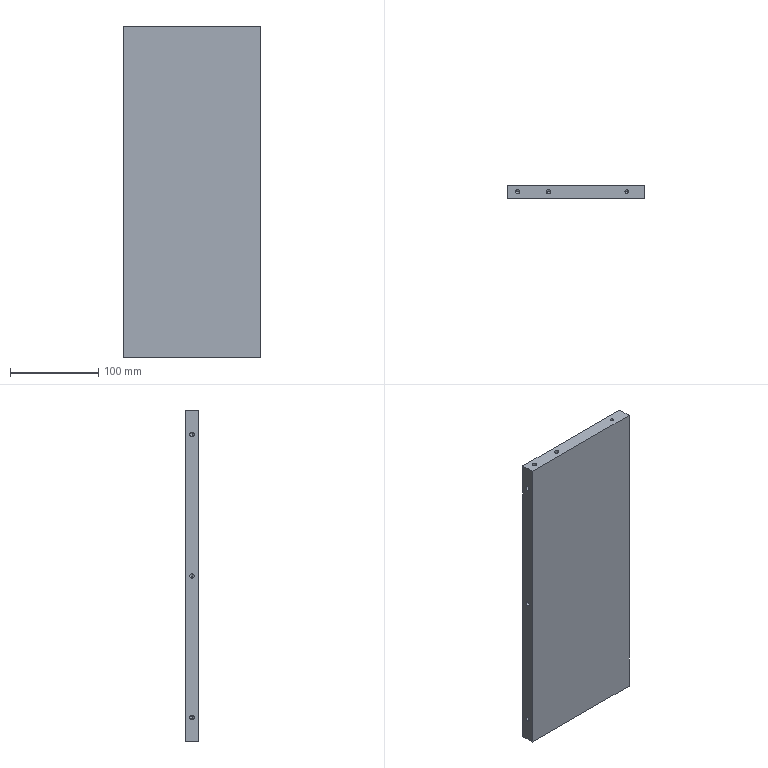Part | STEP file | Left-right side plate | 1 solid | 62 faces | box 155 x 15 x 375 mm | volume 868144 mm3 | cylinder 28 | cone 28 | plane 6 | commonest cylinder face diameters 4.2 x18 5 x10